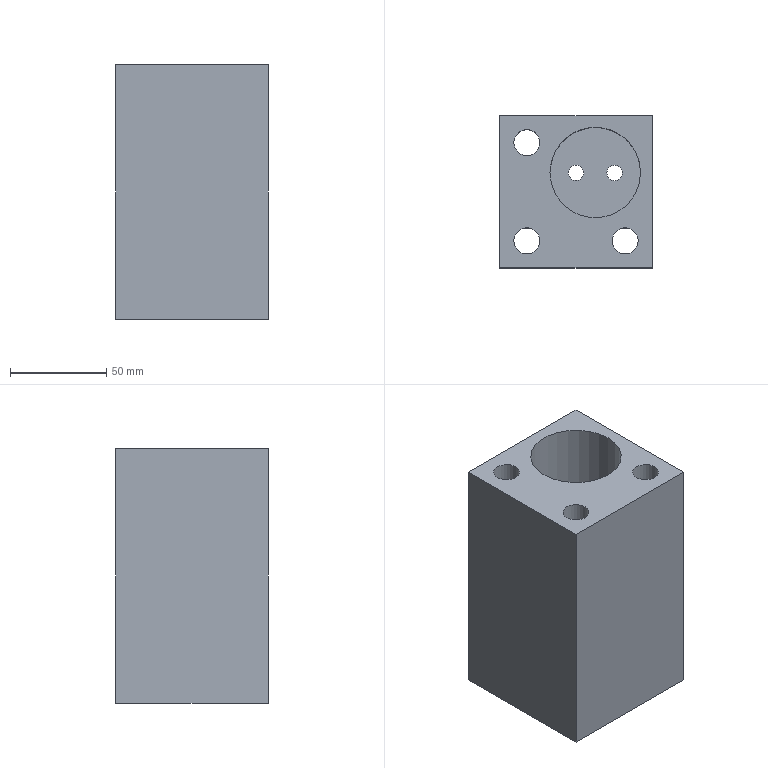Part | STEP file | lll_id4414_x_t | 1 solid | 23 faces | box 79 x 79 x 132 mm | volume 519304 mm3 | plane 12 | cylinder 11 | commonest cylinder face diameters 13.509 x3 20.007 x3 8 x2 13 x2 47 x1
STEP:
#1=CARTESIAN_POINT('',(3455.503,-221.5,-312.));
#2=VERTEX_POINT('',#1);
#3=CARTESIAN_POINT('',(3445.5,-221.5,-312.));
#4=DIRECTION('',(0.,0.,1.));
#5=DIRECTION('',(1.,0.,0.));
#6=AXIS2_PLACEMENT_3D('',#3,#4,#5);
#7=CIRCLE('',#6,10.004);
#8=EDGE_CURVE('',#2,#2,#7,.T.);
#9=ORIENTED_EDGE('',*,*,#8,.T.);
#10=EDGE_LOOP('',(#9));
#11=FACE_BOUND('',#10,.T.);
#12=CARTESIAN_POINT('',(3404.503,-221.5,-312.));
#13=VERTEX_POINT('',#12);
#14=CARTESIAN_POINT('',(3394.5,-221.5,-312.));
#15=DIRECTION('',(0.,0.,1.));
#16=DIRECTION('',(1.,0.,0.));
#17=AXIS2_PLACEMENT_3D('',#14,#15,#16);
#18=CIRCLE('',#17,10.004);
#19=EDGE_CURVE('',#13,#13,#18,.T.);
#20=ORIENTED_EDGE('',*,*,#19,.T.);
#21=EDGE_LOOP('',(#20));
#22=FACE_BOUND('',#21,.T.);
#23=CARTESIAN_POINT('',(3459.5,-156.5,-312.));
#24=VERTEX_POINT('',#23);
#25=CARTESIAN_POINT('',(3380.5,-156.5,-312.));
#26=VERTEX_POINT('',#25);
#27=CARTESIAN_POINT('',(3420.,-156.5,-312.));
#28=DIRECTION('',(-1.,0.,0.));
#29=VECTOR('',#28,1.);
#30=LINE('',#27,#29);
#31=EDGE_CURVE('',#24,#26,#30,.T.);
#32=ORIENTED_EDGE('',*,*,#31,.F.);
#33=CARTESIAN_POINT('',(3459.5,-235.5,-312.));
#34=VERTEX_POINT('',#33);
#35=CARTESIAN_POINT('',(3459.5,-196.,-312.));
#36=DIRECTION('',(0.,1.,0.));
#37=VECTOR('',#36,1.);
#38=LINE('',#35,#37);
#39=EDGE_CURVE('',#34,#24,#38,.T.);
#40=ORIENTED_EDGE('',*,*,#39,.F.);
#41=CARTESIAN_POINT('',(3380.5,-235.5,-312.));
#42=VERTEX_POINT('',#41);
#43=CARTESIAN_POINT('',(3420.,-235.5,-312.));
#44=DIRECTION('',(1.,0.,0.));
#45=VECTOR('',#44,1.);
#46=LINE('',#43,#45);
#47=EDGE_CURVE('',#42,#34,#46,.T.);
#48=ORIENTED_EDGE('',*,*,#47,.F.);
#49=CARTESIAN_POINT('',(3380.5,-196.,-312.));
#50=DIRECTION('',(0.,-1.,0.));
#51=VECTOR('',#50,1.);
#52=LINE('',#49,#51);
#53=EDGE_CURVE('',#26,#42,#52,.T.);
#54=ORIENTED_EDGE('',*,*,#53,.F.);
#55=EDGE_LOOP('',(#32,#40,#48,#54));
#56=FACE_BOUND('',#55,.T.);
#57=CARTESIAN_POINT('',(3404.503,-170.5,-312.));
#58=VERTEX_POINT('',#57);
#59=CARTESIAN_POINT('',(3394.5,-170.5,-312.));
#60=DIRECTION('',(0.,0.,1.));
#61=DIRECTION('',(1.,0.,0.));
#62=AXIS2_PLACEMENT_3D('',#59,#60,#61);
#63=CIRCLE('',#62,10.004);
#64=EDGE_CURVE('',#58,#58,#63,.T.);
#65=ORIENTED_EDGE('',*,*,#64,.T.);
#66=EDGE_LOOP('',(#65));
#67=FACE_BOUND('',#66,.T.);
#68=CARTESIAN_POINT('',(3413.5,-186.,-312.));
#69=VERTEX_POINT('',#68);
#70=CARTESIAN_POINT('',(3420.,-186.,-312.));
#71=DIRECTION('',(0.,0.,-1.));
#72=DIRECTION('',(-1.,0.,0.));
#73=AXIS2_PLACEMENT_3D('',#70,#71,#72);
#74=CIRCLE('',#73,6.5);
#75=EDGE_CURVE('',#69,#69,#74,.T.);
#76=ORIENTED_EDGE('',*,*,#75,.F.);
#77=EDGE_LOOP('',(#76));
#78=FACE_BOUND('',#77,.T.);
#79=CARTESIAN_POINT('',(3433.5,-186.,-312.));
#80=VERTEX_POINT('',#79);
#81=CARTESIAN_POINT('',(3440.,-186.,-312.));
#82=DIRECTION('',(0.,0.,1.));
#83=DIRECTION('',(-1.,0.,0.));
#84=AXIS2_PLACEMENT_3D('',#81,#82,#83);
#85=CIRCLE('',#84,6.5);
#86=EDGE_CURVE('',#80,#80,#85,.T.);
#87=ORIENTED_EDGE('',*,*,#86,.T.);
#88=EDGE_LOOP('',(#87));
#89=FACE_BOUND('',#88,.T.);
#90=CARTESIAN_POINT('',(3420.,-196.,-312.));
#91=DIRECTION('',(0.,0.,-1.));
#92=DIRECTION('',(-1.,0.,0.));
#93=AXIS2_PLACEMENT_3D('',#90,#91,#92);
#94=PLANE('',#93);
#95=ADVANCED_FACE('',(#11,#22,#56,#67,#78,#89),#94,.T.);
#96=CARTESIAN_POINT('',(3436.,-186.,-292.));
#97=VERTEX_POINT('',#96);
#98=CARTESIAN_POINT('',(3440.,-186.,-292.));
#99=DIRECTION('',(0.,0.,-1.));
#100=DIRECTION('',(-1.,0.,0.));
#101=AXIS2_PLACEMENT_3D('',#98,#99,#100);
#102=CIRCLE('',#101,4.);
#103=EDGE_CURVE('',#97,#97,#102,.T.);
#104=ORIENTED_EDGE('',*,*,#103,.F.);
#105=EDGE_LOOP('',(#104));
#106=FACE_BOUND('',#105,.T.);
#107=CARTESIAN_POINT('',(3436.,-186.,-302.));
#108=VERTEX_POINT('',#107);
#109=CARTESIAN_POINT('',(3440.,-186.,-302.));
#110=DIRECTION('',(0.,0.,-1.));
#111=DIRECTION('',(-1.,0.,0.));
#112=AXIS2_PLACEMENT_3D('',#109,#110,#111);
#113=CIRCLE('',#112,4.);
#114=EDGE_CURVE('',#108,#108,#113,.T.);
#115=ORIENTED_EDGE('',*,*,#114,.T.);
#116=EDGE_LOOP('',(#115));
#117=FACE_BOUND('',#116,.T.);
#118=CARTESIAN_POINT('',(3440.,-186.,-404.));
#119=DIRECTION('',(0.,0.,1.));
#120=DIRECTION('',(1.,0.,0.));
#121=AXIS2_PLACEMENT_3D('',#118,#119,#120);
#122=CYLINDRICAL_SURFACE('',#121,4.);
#123=ADVANCED_FACE('',(#106,#117),#122,.F.);
#124=ORIENTED_EDGE('',*,*,#103,.T.);
#125=EDGE_LOOP('',(#124));
#126=FACE_BOUND('',#125,.T.);
#127=CARTESIAN_POINT('',(3406.5,-186.,-292.));
#128=VERTEX_POINT('',#127);
#129=CARTESIAN_POINT('',(3430.,-186.,-292.));
#130=DIRECTION('',(0.,0.,1.));
#131=DIRECTION('',(-1.,0.,0.));
#132=AXIS2_PLACEMENT_3D('',#129,#130,#131);
#133=CIRCLE('',#132,23.5);
#134=EDGE_CURVE('',#128,#128,#133,.T.);
#135=ORIENTED_EDGE('',*,*,#134,.T.);
#136=EDGE_LOOP('',(#135));
#137=FACE_BOUND('',#136,.T.);
#138=CARTESIAN_POINT('',(3416.,-186.,-292.));
#139=VERTEX_POINT('',#138);
#140=CARTESIAN_POINT('',(3420.,-186.,-292.));
#141=DIRECTION('',(0.,0.,1.));
#142=DIRECTION('',(-1.,0.,0.));
#143=AXIS2_PLACEMENT_3D('',#140,#141,#142);
#144=CIRCLE('',#143,4.);
#145=EDGE_CURVE('',#139,#139,#144,.T.);
#146=ORIENTED_EDGE('',*,*,#145,.F.);
#147=EDGE_LOOP('',(#146));
#148=FACE_BOUND('',#147,.T.);
#149=CARTESIAN_POINT('',(3440.8,-186.,-292.));
#150=DIRECTION('',(0.,0.,-1.));
#151=DIRECTION('',(1.,0.,0.));
#152=AXIS2_PLACEMENT_3D('',#149,#150,#151);
#153=PLANE('',#152);
#154=ADVANCED_FACE('',(#126,#137,#148),#153,.F.);
#155=CARTESIAN_POINT('',(3387.745,-170.5,-180.));
#156=VERTEX_POINT('',#155);
#157=CARTESIAN_POINT('',(3394.5,-170.5,-180.));
#158=DIRECTION('',(0.,0.,1.));
#159=DIRECTION('',(-1.,0.,0.));
#160=AXIS2_PLACEMENT_3D('',#157,#158,#159);
#161=CIRCLE('',#160,6.755);
#162=EDGE_CURVE('',#156,#156,#161,.T.);
#163=ORIENTED_EDGE('',*,*,#162,.F.);
#164=EDGE_LOOP('',(#163));
#165=FACE_BOUND('',#164,.T.);
#166=CARTESIAN_POINT('',(3438.745,-221.5,-180.));
#167=VERTEX_POINT('',#166);
#168=CARTESIAN_POINT('',(3445.5,-221.5,-180.));
#169=DIRECTION('',(0.,0.,1.));
#170=DIRECTION('',(-1.,0.,0.));
#171=AXIS2_PLACEMENT_3D('',#168,#169,#170);
#172=CIRCLE('',#171,6.755);
#173=EDGE_CURVE('',#167,#167,#172,.T.);
#174=ORIENTED_EDGE('',*,*,#173,.F.);
#175=EDGE_LOOP('',(#174));
#176=FACE_BOUND('',#175,.T.);
#177=CARTESIAN_POINT('',(3387.745,-221.5,-180.));
#178=VERTEX_POINT('',#177);
#179=CARTESIAN_POINT('',(3394.5,-221.5,-180.));
#180=DIRECTION('',(0.,0.,1.));
#181=DIRECTION('',(-1.,0.,0.));
#182=AXIS2_PLACEMENT_3D('',#179,#180,#181);
#183=CIRCLE('',#182,6.755);
#184=EDGE_CURVE('',#178,#178,#183,.T.);
#185=ORIENTED_EDGE('',*,*,#184,.F.);
#186=EDGE_LOOP('',(#185));
#187=FACE_BOUND('',#186,.T.);
#188=CARTESIAN_POINT('',(3406.5,-186.,-180.));
#189=VERTEX_POINT('',#188);
#190=CARTESIAN_POINT('',(3430.,-186.,-180.));
#191=DIRECTION('',(0.,0.,1.));
#192=DIRECTION('',(-1.,0.,0.));
#193=AXIS2_PLACEMENT_3D('',#190,#191,#192);
#194=CIRCLE('',#193,23.5);
#195=EDGE_CURVE('',#189,#189,#194,.T.);
#196=ORIENTED_EDGE('',*,*,#195,.F.);
#197=EDGE_LOOP('',(#196));
#198=FACE_BOUND('',#197,.T.);
#199=CARTESIAN_POINT('',(3459.5,-156.5,-180.));
#200=VERTEX_POINT('',#199);
#201=CARTESIAN_POINT('',(3459.5,-235.5,-180.));
#202=VERTEX_POINT('',#201);
#203=CARTESIAN_POINT('',(3459.5,-196.,-180.));
#204=DIRECTION('',(0.,-1.,0.));
#205=VECTOR('',#204,1.);
#206=LINE('',#203,#205);
#207=EDGE_CURVE('',#200,#202,#206,.T.);
#208=ORIENTED_EDGE('',*,*,#207,.F.);
#209=CARTESIAN_POINT('',(3380.5,-156.5,-180.));
#210=VERTEX_POINT('',#209);
#211=CARTESIAN_POINT('',(3420.,-156.5,-180.));
#212=DIRECTION('',(1.,0.,0.));
#213=VECTOR('',#212,1.);
#214=LINE('',#211,#213);
#215=EDGE_CURVE('',#210,#200,#214,.T.);
#216=ORIENTED_EDGE('',*,*,#215,.F.);
#217=CARTESIAN_POINT('',(3380.5,-235.5,-180.));
#218=VERTEX_POINT('',#217);
#219=CARTESIAN_POINT('',(3380.5,-196.,-180.));
#220=DIRECTION('',(0.,1.,0.));
#221=VECTOR('',#220,1.);
#222=LINE('',#219,#221);
#223=EDGE_CURVE('',#218,#210,#222,.T.);
#224=ORIENTED_EDGE('',*,*,#223,.F.);
#225=CARTESIAN_POINT('',(3420.,-235.5,-180.));
#226=DIRECTION('',(-1.,0.,0.));
#227=VECTOR('',#226,1.);
#228=LINE('',#225,#227);
#229=EDGE_CURVE('',#202,#218,#228,.T.);
#230=ORIENTED_EDGE('',*,*,#229,.F.);
#231=EDGE_LOOP('',(#208,#216,#224,#230));
#232=FACE_BOUND('',#231,.T.);
#233=CARTESIAN_POINT('',(2432.435,-387.,-180.));
#234=DIRECTION('',(0.,0.,-1.));
#235=DIRECTION('',(-1.,0.,0.));
#236=AXIS2_PLACEMENT_3D('',#233,#234,#235);
#237=PLANE('',#236);
#238=ADVANCED_FACE('',(#165,#176,#187,#198,#232),#237,.F.);
#239=CARTESIAN_POINT('',(3459.5,-235.5,-312.));
#240=DIRECTION('',(0.,0.,1.));
#241=VECTOR('',#240,1.);
#242=LINE('',#239,#241);
#243=EDGE_CURVE('',#34,#202,#242,.T.);
#244=ORIENTED_EDGE('',*,*,#243,.T.);
#245=ORIENTED_EDGE('',*,*,#229,.T.);
#246=CARTESIAN_POINT('',(3380.5,-235.5,-312.));
#247=DIRECTION('',(0.,0.,1.));
#248=VECTOR('',#247,1.);
#249=LINE('',#246,#248);
#250=EDGE_CURVE('',#42,#218,#249,.T.);
#251=ORIENTED_EDGE('',*,*,#250,.F.);
#252=ORIENTED_EDGE('',*,*,#47,.T.);
#253=EDGE_LOOP('',(#244,#245,#251,#252));
#254=FACE_OUTER_BOUND('',#253,.T.);
#255=CARTESIAN_POINT('',(3420.,-235.5,-312.));
#256=DIRECTION('',(0.,-1.,0.));
#257=DIRECTION('',(0.,0.,-1.));
#258=AXIS2_PLACEMENT_3D('',#255,#256,#257);
#259=PLANE('',#258);
#260=ADVANCED_FACE('',(#254),#259,.T.);
#261=ORIENTED_EDGE('',*,*,#250,.T.);
#262=ORIENTED_EDGE('',*,*,#223,.T.);
#263=CARTESIAN_POINT('',(3380.5,-156.5,-312.));
#264=DIRECTION('',(0.,0.,1.));
#265=VECTOR('',#264,1.);
#266=LINE('',#263,#265);
#267=EDGE_CURVE('',#26,#210,#266,.T.);
#268=ORIENTED_EDGE('',*,*,#267,.F.);
#269=ORIENTED_EDGE('',*,*,#53,.T.);
#270=EDGE_LOOP('',(#261,#262,#268,#269));
#271=FACE_OUTER_BOUND('',#270,.T.);
#272=CARTESIAN_POINT('',(3380.5,-196.,-312.));
#273=DIRECTION('',(-1.,0.,0.));
#274=DIRECTION('',(0.,0.,1.));
#275=AXIS2_PLACEMENT_3D('',#272,#273,#274);
#276=PLANE('',#275);
#277=ADVANCED_FACE('',(#271),#276,.T.);
#278=ORIENTED_EDGE('',*,*,#215,.T.);
#279=CARTESIAN_POINT('',(3459.5,-156.5,-312.));
#280=DIRECTION('',(0.,0.,-1.));
#281=VECTOR('',#280,1.);
#282=LINE('',#279,#281);
#283=EDGE_CURVE('',#200,#24,#282,.T.);
#284=ORIENTED_EDGE('',*,*,#283,.T.);
#285=ORIENTED_EDGE('',*,*,#31,.T.);
#286=ORIENTED_EDGE('',*,*,#267,.T.);
#287=EDGE_LOOP('',(#278,#284,#285,#286));
#288=FACE_OUTER_BOUND('',#287,.T.);
#289=CARTESIAN_POINT('',(3420.,-156.5,-312.));
#290=DIRECTION('',(0.,1.,0.));
#291=DIRECTION('',(0.,0.,1.));
#292=AXIS2_PLACEMENT_3D('',#289,#290,#291);
#293=PLANE('',#292);
#294=ADVANCED_FACE('',(#288),#293,.T.);
#295=ORIENTED_EDGE('',*,*,#39,.T.);
#296=ORIENTED_EDGE('',*,*,#283,.F.);
#297=ORIENTED_EDGE('',*,*,#207,.T.);
#298=ORIENTED_EDGE('',*,*,#243,.F.);
#299=EDGE_LOOP('',(#295,#296,#297,#298));
#300=FACE_OUTER_BOUND('',#299,.T.);
#301=CARTESIAN_POINT('',(3459.5,-196.,-312.));
#302=DIRECTION('',(1.,0.,0.));
#303=DIRECTION('',(0.,0.,-1.));
#304=AXIS2_PLACEMENT_3D('',#301,#302,#303);
#305=PLANE('',#304);
#306=ADVANCED_FACE('',(#300),#305,.T.);
#307=ORIENTED_EDGE('',*,*,#134,.F.);
#308=EDGE_LOOP('',(#307));
#309=FACE_BOUND('',#308,.T.);
#310=ORIENTED_EDGE('',*,*,#195,.T.);
#311=EDGE_LOOP('',(#310));
#312=FACE_BOUND('',#311,.T.);
#313=CARTESIAN_POINT('',(3430.,-186.,-292.));
#314=DIRECTION('',(0.,0.,1.));
#315=DIRECTION('',(1.,0.,0.));
#316=AXIS2_PLACEMENT_3D('',#313,#314,#315);
#317=CYLINDRICAL_SURFACE('',#316,23.5);
#318=ADVANCED_FACE('',(#309,#312),#317,.F.);
#319=ORIENTED_EDGE('',*,*,#184,.T.);
#320=EDGE_LOOP('',(#319));
#321=FACE_BOUND('',#320,.T.);
#322=CARTESIAN_POINT('',(3401.255,-221.5,-215.));
#323=VERTEX_POINT('',#322);
#324=CARTESIAN_POINT('',(3394.5,-221.5,-215.));
#325=DIRECTION('',(0.,0.,1.));
#326=DIRECTION('',(1.,0.,0.));
#327=AXIS2_PLACEMENT_3D('',#324,#325,#326);
#328=CIRCLE('',#327,6.755);
#329=EDGE_CURVE('',#323,#323,#328,.T.);
#330=ORIENTED_EDGE('',*,*,#329,.F.);
#331=EDGE_LOOP('',(#330));
#332=FACE_BOUND('',#331,.T.);
#333=CARTESIAN_POINT('',(3394.5,-221.5,-317.));
#334=DIRECTION('',(0.,0.,1.));
#335=DIRECTION('',(1.,0.,0.));
#336=AXIS2_PLACEMENT_3D('',#333,#334,#335);
#337=CYLINDRICAL_SURFACE('',#336,6.755);
#338=ADVANCED_FACE('',(#321,#332),#337,.F.);
#339=ORIENTED_EDGE('',*,*,#329,.T.);
#340=EDGE_LOOP('',(#339));
#341=FACE_BOUND('',#340,.T.);
#342=CARTESIAN_POINT('',(3404.503,-221.5,-215.));
#343=VERTEX_POINT('',#342);
#344=CARTESIAN_POINT('',(3394.5,-221.5,-215.));
#345=DIRECTION('',(0.,0.,1.));
#346=DIRECTION('',(1.,0.,0.));
#347=AXIS2_PLACEMENT_3D('',#344,#345,#346);
#348=CIRCLE('',#347,10.004);
#349=EDGE_CURVE('',#343,#343,#348,.T.);
#350=ORIENTED_EDGE('',*,*,#349,.F.);
#351=EDGE_LOOP('',(#350));
#352=FACE_BOUND('',#351,.T.);
#353=CARTESIAN_POINT('',(3394.5,-221.5,-215.));
#354=DIRECTION('',(0.,0.,1.));
#355=DIRECTION('',(1.,0.,0.));
#356=AXIS2_PLACEMENT_3D('',#353,#354,#355);
#357=PLANE('',#356);
#358=ADVANCED_FACE('',(#341,#352),#357,.F.);
#359=ORIENTED_EDGE('',*,*,#349,.T.);
#360=EDGE_LOOP('',(#359));
#361=FACE_BOUND('',#360,.T.);
#362=ORIENTED_EDGE('',*,*,#19,.F.);
#363=EDGE_LOOP('',(#362));
#364=FACE_BOUND('',#363,.T.);
#365=CARTESIAN_POINT('',(3394.5,-221.5,-312.));
#366=DIRECTION('',(0.,0.,1.));
#367=DIRECTION('',(1.,0.,0.));
#368=AXIS2_PLACEMENT_3D('',#365,#366,#367);
#369=CYLINDRICAL_SURFACE('',#368,10.004);
#370=ADVANCED_FACE('',(#361,#364),#369,.F.);
#371=ORIENTED_EDGE('',*,*,#173,.T.);
#372=EDGE_LOOP('',(#371));
#373=FACE_BOUND('',#372,.T.);
#374=CARTESIAN_POINT('',(3452.255,-221.5,-215.));
#375=VERTEX_POINT('',#374);
#376=CARTESIAN_POINT('',(3445.5,-221.5,-215.));
#377=DIRECTION('',(0.,0.,1.));
#378=DIRECTION('',(1.,0.,0.));
#379=AXIS2_PLACEMENT_3D('',#376,#377,#378);
#380=CIRCLE('',#379,6.755);
#381=EDGE_CURVE('',#375,#375,#380,.T.);
#382=ORIENTED_EDGE('',*,*,#381,.F.);
#383=EDGE_LOOP('',(#382));
#384=FACE_BOUND('',#383,.T.);
#385=CARTESIAN_POINT('',(3445.5,-221.5,-317.));
#386=DIRECTION('',(0.,0.,1.));
#387=DIRECTION('',(1.,0.,0.));
#388=AXIS2_PLACEMENT_3D('',#385,#386,#387);
#389=CYLINDRICAL_SURFACE('',#388,6.755);
#390=ADVANCED_FACE('',(#373,#384),#389,.F.);
#391=ORIENTED_EDGE('',*,*,#381,.T.);
#392=EDGE_LOOP('',(#391));
#393=FACE_BOUND('',#392,.T.);
#394=CARTESIAN_POINT('',(3455.503,-221.5,-215.));
#395=VERTEX_POINT('',#394);
#396=CARTESIAN_POINT('',(3445.5,-221.5,-215.));
#397=DIRECTION('',(0.,0.,1.));
#398=DIRECTION('',(1.,0.,0.));
#399=AXIS2_PLACEMENT_3D('',#396,#397,#398);
#400=CIRCLE('',#399,10.004);
#401=EDGE_CURVE('',#395,#395,#400,.T.);
#402=ORIENTED_EDGE('',*,*,#401,.F.);
#403=EDGE_LOOP('',(#402));
#404=FACE_BOUND('',#403,.T.);
#405=CARTESIAN_POINT('',(3445.5,-221.5,-215.));
#406=DIRECTION('',(0.,0.,1.));
#407=DIRECTION('',(1.,0.,0.));
#408=AXIS2_PLACEMENT_3D('',#405,#406,#407);
#409=PLANE('',#408);
#410=ADVANCED_FACE('',(#393,#404),#409,.F.);
#411=ORIENTED_EDGE('',*,*,#401,.T.);
#412=EDGE_LOOP('',(#411));
#413=FACE_BOUND('',#412,.T.);
#414=ORIENTED_EDGE('',*,*,#8,.F.);
#415=EDGE_LOOP('',(#414));
#416=FACE_BOUND('',#415,.T.);
#417=CARTESIAN_POINT('',(3445.5,-221.5,-312.));
#418=DIRECTION('',(0.,0.,1.));
#419=DIRECTION('',(1.,0.,0.));
#420=AXIS2_PLACEMENT_3D('',#417,#418,#419);
#421=CYLINDRICAL_SURFACE('',#420,10.004);
#422=ADVANCED_FACE('',(#413,#416),#421,.F.);
#423=ORIENTED_EDGE('',*,*,#162,.T.);
#424=EDGE_LOOP('',(#423));
#425=FACE_BOUND('',#424,.T.);
#426=CARTESIAN_POINT('',(3401.255,-170.5,-215.));
#427=VERTEX_POINT('',#426);
#428=CARTESIAN_POINT('',(3394.5,-170.5,-215.));
#429=DIRECTION('',(0.,0.,1.));
#430=DIRECTION('',(1.,0.,0.));
#431=AXIS2_PLACEMENT_3D('',#428,#429,#430);
#432=CIRCLE('',#431,6.755);
#433=EDGE_CURVE('',#427,#427,#432,.T.);
#434=ORIENTED_EDGE('',*,*,#433,.F.);
#435=EDGE_LOOP('',(#434));
#436=FACE_BOUND('',#435,.T.);
#437=CARTESIAN_POINT('',(3394.5,-170.5,-317.));
#438=DIRECTION('',(0.,0.,1.));
#439=DIRECTION('',(1.,0.,0.));
#440=AXIS2_PLACEMENT_3D('',#437,#438,#439);
#441=CYLINDRICAL_SURFACE('',#440,6.755);
#442=ADVANCED_FACE('',(#425,#436),#441,.F.);
#443=ORIENTED_EDGE('',*,*,#433,.T.);
#444=EDGE_LOOP('',(#443));
#445=FACE_BOUND('',#444,.T.);
#446=CARTESIAN_POINT('',(3404.503,-170.5,-215.));
#447=VERTEX_POINT('',#446);
#448=CARTESIAN_POINT('',(3394.5,-170.5,-215.));
#449=DIRECTION('',(0.,0.,1.));
#450=DIRECTION('',(1.,0.,0.));
#451=AXIS2_PLACEMENT_3D('',#448,#449,#450);
#452=CIRCLE('',#451,10.004);
#453=EDGE_CURVE('',#447,#447,#452,.T.);
#454=ORIENTED_EDGE('',*,*,#453,.F.);
#455=EDGE_LOOP('',(#454));
#456=FACE_BOUND('',#455,.T.);
#457=CARTESIAN_POINT('',(3394.5,-170.5,-215.));
#458=DIRECTION('',(0.,0.,1.));
#459=DIRECTION('',(1.,0.,0.));
#460=AXIS2_PLACEMENT_3D('',#457,#458,#459);
#461=PLANE('',#460);
#462=ADVANCED_FACE('',(#445,#456),#461,.F.);
#463=ORIENTED_EDGE('',*,*,#453,.T.);
#464=EDGE_LOOP('',(#463));
#465=FACE_BOUND('',#464,.T.);
#466=ORIENTED_EDGE('',*,*,#64,.F.);
#467=EDGE_LOOP('',(#466));
#468=FACE_BOUND('',#467,.T.);
#469=CARTESIAN_POINT('',(3394.5,-170.5,-312.));
#470=DIRECTION('',(0.,0.,1.));
#471=DIRECTION('',(1.,0.,0.));
#472=AXIS2_PLACEMENT_3D('',#469,#470,#471);
#473=CYLINDRICAL_SURFACE('',#472,10.004);
#474=ADVANCED_FACE('',(#465,#468),#473,.F.);
#475=CARTESIAN_POINT('',(3424.,-186.,-302.));
#476=VERTEX_POINT('',#475);
#477=CARTESIAN_POINT('',(3420.,-186.,-302.));
#478=DIRECTION('',(0.,0.,-1.));
#479=DIRECTION('',(1.,0.,0.));
#480=AXIS2_PLACEMENT_3D('',#477,#478,#479);
#481=CIRCLE('',#480,4.);
#482=EDGE_CURVE('',#476,#476,#481,.T.);
#483=ORIENTED_EDGE('',*,*,#482,.T.);
#484=EDGE_LOOP('',(#483));
#485=FACE_BOUND('',#484,.T.);
#486=ORIENTED_EDGE('',*,*,#145,.T.);
#487=EDGE_LOOP('',(#486));
#488=FACE_BOUND('',#487,.T.);
#489=CARTESIAN_POINT('',(3420.,-186.,-404.));
#490=DIRECTION('',(0.,0.,1.));
#491=DIRECTION('',(1.,0.,0.));
#492=AXIS2_PLACEMENT_3D('',#489,#490,#491);
#493=CYLINDRICAL_SURFACE('',#492,4.);
#494=ADVANCED_FACE('',(#485,#488),#493,.F.);
#495=CARTESIAN_POINT('',(3426.5,-186.,-302.));
#496=VERTEX_POINT('',#495);
#497=CARTESIAN_POINT('',(3420.,-186.,-302.));
#498=DIRECTION('',(0.,0.,-1.));
#499=DIRECTION('',(1.,0.,0.));
#500=AXIS2_PLACEMENT_3D('',#497,#498,#499);
#501=CIRCLE('',#500,6.5);
#502=EDGE_CURVE('',#496,#496,#501,.T.);
#503=ORIENTED_EDGE('',*,*,#502,.T.);
#504=EDGE_LOOP('',(#503));
#505=FACE_BOUND('',#504,.T.);
#506=ORIENTED_EDGE('',*,*,#482,.F.);
#507=EDGE_LOOP('',(#506));
#508=FACE_BOUND('',#507,.T.);
#509=CARTESIAN_POINT('',(3420.,-186.,-302.));
#510=DIRECTION('',(0.,0.,1.));
#511=DIRECTION('',(1.,0.,0.));
#512=AXIS2_PLACEMENT_3D('',#509,#510,#511);
#513=PLANE('',#512);
#514=ADVANCED_FACE('',(#505,#508),#513,.F.);
#515=ORIENTED_EDGE('',*,*,#75,.T.);
#516=EDGE_LOOP('',(#515));
#517=FACE_BOUND('',#516,.T.);
#518=ORIENTED_EDGE('',*,*,#502,.F.);
#519=EDGE_LOOP('',(#518));
#520=FACE_BOUND('',#519,.T.);
#521=CARTESIAN_POINT('',(3420.,-186.,-404.));
#522=DIRECTION('',(0.,0.,1.));
#523=DIRECTION('',(1.,0.,0.));
#524=AXIS2_PLACEMENT_3D('',#521,#522,#523);
#525=CYLINDRICAL_SURFACE('',#524,6.5);
#526=ADVANCED_FACE('',(#517,#520),#525,.F.);
#527=ORIENTED_EDGE('',*,*,#86,.F.);
#528=EDGE_LOOP('',(#527));
#529=FACE_BOUND('',#528,.T.);
#530=CARTESIAN_POINT('',(3433.5,-186.,-302.));
#531=VERTEX_POINT('',#530);
#532=CARTESIAN_POINT('',(3440.,-186.,-302.));
#533=DIRECTION('',(0.,0.,1.));
#534=DIRECTION('',(-1.,0.,0.));
#535=AXIS2_PLACEMENT_3D('',#532,#533,#534);
#536=CIRCLE('',#535,6.5);
#537=EDGE_CURVE('',#531,#531,#536,.T.);
#538=ORIENTED_EDGE('',*,*,#537,.T.);
#539=EDGE_LOOP('',(#538));
#540=FACE_BOUND('',#539,.T.);
#541=CARTESIAN_POINT('',(3440.,-186.,-404.));
#542=DIRECTION('',(0.,0.,1.));
#543=DIRECTION('',(1.,0.,0.));
#544=AXIS2_PLACEMENT_3D('',#541,#542,#543);
#545=CYLINDRICAL_SURFACE('',#544,6.5);
#546=ADVANCED_FACE('',(#529,#540),#545,.F.);
#547=ORIENTED_EDGE('',*,*,#114,.F.);
#548=EDGE_LOOP('',(#547));
#549=FACE_BOUND('',#548,.T.);
#550=ORIENTED_EDGE('',*,*,#537,.F.);
#551=EDGE_LOOP('',(#550));
#552=FACE_BOUND('',#551,.T.);
#553=CARTESIAN_POINT('',(3440.,-186.,-302.));
#554=DIRECTION('',(0.,0.,-1.));
#555=DIRECTION('',(-1.,0.,0.));
#556=AXIS2_PLACEMENT_3D('',#553,#554,#555);
#557=PLANE('',#556);
#558=ADVANCED_FACE('',(#549,#552),#557,.T.);
#559=CLOSED_SHELL('',(#95,#123,#154,#238,#260,#277,#294,#306,#318,#338,#358,#370,#390,#410,#422,#442,#462,#474,#494,#514,#526,#546,#558));
#560=MANIFOLD_SOLID_BREP('',#559);
#561=(LENGTH_UNIT()NAMED_UNIT(*)SI_UNIT(.MILLI.,.METRE.));
#562=UNCERTAINTY_MEASURE_WITH_UNIT(LENGTH_MEASURE(0.00002),#561,'','');
#563=(NAMED_UNIT(*)PLANE_ANGLE_UNIT()SI_UNIT($,.RADIAN.));
#564=PLANE_ANGLE_MEASURE_WITH_UNIT(PLANE_ANGLE_MEASURE(0.01745),#563);
#565=DIMENSIONAL_EXPONENTS(0.,0.,0.,0.,0.,0.,0.);
#566=(CONVERSION_BASED_UNIT('DEGREE',#564)NAMED_UNIT(#565)PLANE_ANGLE_UNIT());
#567=(NAMED_UNIT(*)SI_UNIT($,.STERADIAN.)SOLID_ANGLE_UNIT());
#568=(GEOMETRIC_REPRESENTATION_CONTEXT(3)GLOBAL_UNCERTAINTY_ASSIGNED_CONTEXT((#562))GLOBAL_UNIT_ASSIGNED_CONTEXT((#561,#566,#567))REPRESENTATION_CONTEXT('',''));
#569=ADVANCED_BREP_SHAPE_REPRESENTATION('',(#560),#568);